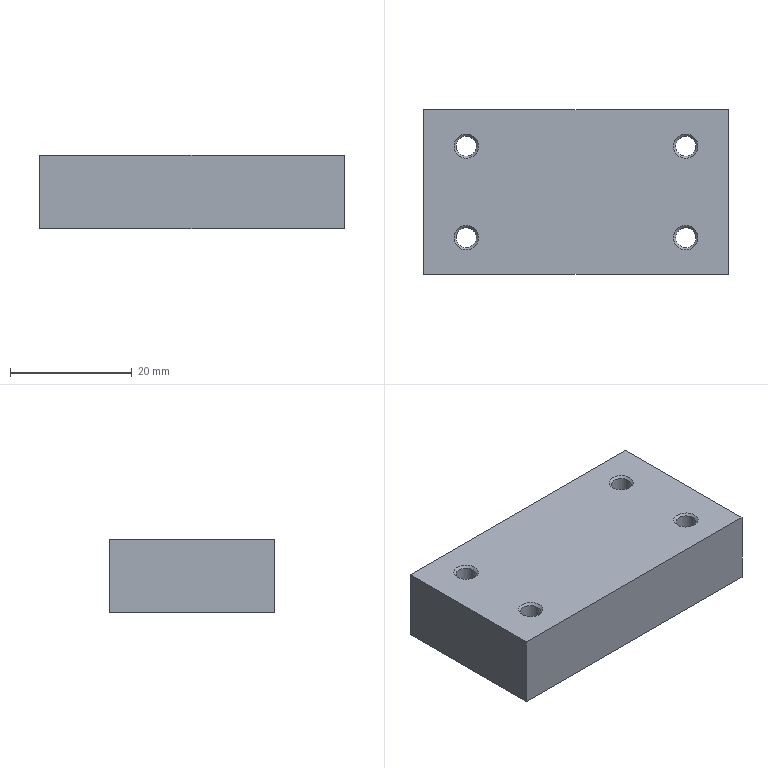Part | NX | features SIMPLE HOLE 4, SYMBOLIC_THREAD 4, DATUM_CSYS 2, BLOCK 1, HOLE PACKAGE 1, SKETCH 1 | 1 solid | 18 faces | box 50 x 27 x 12 mm | volume 15784 mm3 | cone 8 | plane 6 | cylinder 4 | commonest cylinder face diameters 3.3 x4
STEP:
#1=CARTESIAN_POINT('',(45.,21.,12.));
#2=VERTEX_POINT('',#1);
#3=CARTESIAN_POINT('',(43.,21.,12.));
#4=DIRECTION('',(0.,0.,1.));
#5=DIRECTION('',(1.,0.,0.));
#6=AXIS2_PLACEMENT_3D('',#3,#4,#5);
#7=CIRCLE('',#6,2.);
#8=EDGE_CURVE('',#2,#2,#7,.F.);
#9=ORIENTED_EDGE('',*,*,#8,.T.);
#10=EDGE_LOOP('',(#9));
#11=FACE_BOUND('',#10,.T.);
#12=CARTESIAN_POINT('',(45.,6.,12.));
#13=VERTEX_POINT('',#12);
#14=CARTESIAN_POINT('',(43.,6.,12.));
#15=DIRECTION('',(0.,0.,1.));
#16=DIRECTION('',(1.,0.,0.));
#17=AXIS2_PLACEMENT_3D('',#14,#15,#16);
#18=CIRCLE('',#17,2.);
#19=EDGE_CURVE('',#13,#13,#18,.F.);
#20=ORIENTED_EDGE('',*,*,#19,.T.);
#21=EDGE_LOOP('',(#20));
#22=FACE_BOUND('',#21,.T.);
#23=CARTESIAN_POINT('',(9.,21.,12.));
#24=VERTEX_POINT('',#23);
#25=CARTESIAN_POINT('',(7.,21.,12.));
#26=DIRECTION('',(0.,0.,1.));
#27=DIRECTION('',(1.,0.,0.));
#28=AXIS2_PLACEMENT_3D('',#25,#26,#27);
#29=CIRCLE('',#28,2.);
#30=EDGE_CURVE('',#24,#24,#29,.F.);
#31=ORIENTED_EDGE('',*,*,#30,.T.);
#32=EDGE_LOOP('',(#31));
#33=FACE_BOUND('',#32,.T.);
#34=CARTESIAN_POINT('',(9.,6.,12.));
#35=VERTEX_POINT('',#34);
#36=CARTESIAN_POINT('',(7.,6.,12.));
#37=DIRECTION('',(0.,0.,1.));
#38=DIRECTION('',(1.,0.,0.));
#39=AXIS2_PLACEMENT_3D('',#36,#37,#38);
#40=CIRCLE('',#39,2.);
#41=EDGE_CURVE('',#35,#35,#40,.F.);
#42=ORIENTED_EDGE('',*,*,#41,.T.);
#43=EDGE_LOOP('',(#42));
#44=FACE_BOUND('',#43,.T.);
#45=CARTESIAN_POINT('',(50.,0.,12.));
#46=VERTEX_POINT('',#45);
#47=CARTESIAN_POINT('',(0.,0.,12.));
#48=VERTEX_POINT('',#47);
#49=CARTESIAN_POINT('',(25.,0.,12.));
#50=DIRECTION('',(-1.,0.,0.));
#51=VECTOR('',#50,1000.);
#52=LINE('',#49,#51);
#53=EDGE_CURVE('',#46,#48,#52,.T.);
#54=ORIENTED_EDGE('',*,*,#53,.F.);
#55=CARTESIAN_POINT('',(50.,27.,12.));
#56=VERTEX_POINT('',#55);
#57=CARTESIAN_POINT('',(50.,13.5,12.));
#58=DIRECTION('',(0.,-1.,0.));
#59=VECTOR('',#58,1000.);
#60=LINE('',#57,#59);
#61=EDGE_CURVE('',#56,#46,#60,.T.);
#62=ORIENTED_EDGE('',*,*,#61,.F.);
#63=CARTESIAN_POINT('',(0.,27.,12.));
#64=VERTEX_POINT('',#63);
#65=CARTESIAN_POINT('',(25.,27.,12.));
#66=DIRECTION('',(1.,0.,0.));
#67=VECTOR('',#66,1000.);
#68=LINE('',#65,#67);
#69=EDGE_CURVE('',#64,#56,#68,.T.);
#70=ORIENTED_EDGE('',*,*,#69,.F.);
#71=CARTESIAN_POINT('',(0.,13.5,12.));
#72=DIRECTION('',(0.,1.,0.));
#73=VECTOR('',#72,1000.);
#74=LINE('',#71,#73);
#75=EDGE_CURVE('',#48,#64,#74,.T.);
#76=ORIENTED_EDGE('',*,*,#75,.F.);
#77=EDGE_LOOP('',(#54,#62,#70,#76));
#78=FACE_BOUND('',#77,.T.);
#79=CARTESIAN_POINT('',(25.,13.5,12.));
#80=DIRECTION('',(0.,0.,1.));
#81=DIRECTION('',(1.,0.,0.));
#82=AXIS2_PLACEMENT_3D('',#79,#80,#81);
#83=PLANE('',#82);
#84=ADVANCED_FACE('',(#11,#22,#33,#44,#78),#83,.T.);
#85=CARTESIAN_POINT('',(50.,0.,0.));
#86=VERTEX_POINT('',#85);
#87=CARTESIAN_POINT('',(50.,0.,0.));
#88=DIRECTION('',(0.,0.,1.));
#89=VECTOR('',#88,1000.);
#90=LINE('',#87,#89);
#91=EDGE_CURVE('',#86,#46,#90,.T.);
#92=ORIENTED_EDGE('',*,*,#91,.T.);
#93=ORIENTED_EDGE('',*,*,#53,.T.);
#94=CARTESIAN_POINT('',(0.,0.,0.));
#95=VERTEX_POINT('',#94);
#96=CARTESIAN_POINT('',(0.,0.,0.));
#97=DIRECTION('',(0.,0.,1.));
#98=VECTOR('',#97,1000.);
#99=LINE('',#96,#98);
#100=EDGE_CURVE('',#95,#48,#99,.T.);
#101=ORIENTED_EDGE('',*,*,#100,.F.);
#102=CARTESIAN_POINT('',(25.,0.,0.));
#103=DIRECTION('',(1.,0.,0.));
#104=VECTOR('',#103,1000.);
#105=LINE('',#102,#104);
#106=EDGE_CURVE('',#95,#86,#105,.T.);
#107=ORIENTED_EDGE('',*,*,#106,.T.);
#108=EDGE_LOOP('',(#92,#93,#101,#107));
#109=FACE_BOUND('',#108,.T.);
#110=CARTESIAN_POINT('',(25.,0.,0.));
#111=DIRECTION('',(0.,-1.,0.));
#112=DIRECTION('',(0.,0.,-1.));
#113=AXIS2_PLACEMENT_3D('',#110,#111,#112);
#114=PLANE('',#113);
#115=ADVANCED_FACE('',(#109),#114,.T.);
#116=ORIENTED_EDGE('',*,*,#100,.T.);
#117=ORIENTED_EDGE('',*,*,#75,.T.);
#118=CARTESIAN_POINT('',(0.,27.,0.));
#119=VERTEX_POINT('',#118);
#120=CARTESIAN_POINT('',(0.,27.,0.));
#121=DIRECTION('',(0.,0.,1.));
#122=VECTOR('',#121,1000.);
#123=LINE('',#120,#122);
#124=EDGE_CURVE('',#119,#64,#123,.T.);
#125=ORIENTED_EDGE('',*,*,#124,.F.);
#126=CARTESIAN_POINT('',(0.,13.5,0.));
#127=DIRECTION('',(0.,-1.,0.));
#128=VECTOR('',#127,1000.);
#129=LINE('',#126,#128);
#130=EDGE_CURVE('',#119,#95,#129,.T.);
#131=ORIENTED_EDGE('',*,*,#130,.T.);
#132=EDGE_LOOP('',(#116,#117,#125,#131));
#133=FACE_BOUND('',#132,.T.);
#134=CARTESIAN_POINT('',(0.,13.5,0.));
#135=DIRECTION('',(-1.,0.,0.));
#136=DIRECTION('',(0.,0.,1.));
#137=AXIS2_PLACEMENT_3D('',#134,#135,#136);
#138=PLANE('',#137);
#139=ADVANCED_FACE('',(#133),#138,.T.);
#140=ORIENTED_EDGE('',*,*,#124,.T.);
#141=ORIENTED_EDGE('',*,*,#69,.T.);
#142=CARTESIAN_POINT('',(50.,27.,0.));
#143=VERTEX_POINT('',#142);
#144=CARTESIAN_POINT('',(50.,27.,0.));
#145=DIRECTION('',(0.,0.,1.));
#146=VECTOR('',#145,1000.);
#147=LINE('',#144,#146);
#148=EDGE_CURVE('',#143,#56,#147,.T.);
#149=ORIENTED_EDGE('',*,*,#148,.F.);
#150=CARTESIAN_POINT('',(25.,27.,0.));
#151=DIRECTION('',(-1.,0.,0.));
#152=VECTOR('',#151,1000.);
#153=LINE('',#150,#152);
#154=EDGE_CURVE('',#143,#119,#153,.T.);
#155=ORIENTED_EDGE('',*,*,#154,.T.);
#156=EDGE_LOOP('',(#140,#141,#149,#155));
#157=FACE_BOUND('',#156,.T.);
#158=CARTESIAN_POINT('',(25.,27.,0.));
#159=DIRECTION('',(0.,1.,0.));
#160=DIRECTION('',(0.,0.,1.));
#161=AXIS2_PLACEMENT_3D('',#158,#159,#160);
#162=PLANE('',#161);
#163=ADVANCED_FACE('',(#157),#162,.T.);
#164=CARTESIAN_POINT('',(41.,21.,0.));
#165=VERTEX_POINT('',#164);
#166=CARTESIAN_POINT('',(43.,21.,0.));
#167=DIRECTION('',(0.,0.,-1.));
#168=DIRECTION('',(-1.,0.,0.));
#169=AXIS2_PLACEMENT_3D('',#166,#167,#168);
#170=CIRCLE('',#169,2.);
#171=EDGE_CURVE('',#165,#165,#170,.F.);
#172=ORIENTED_EDGE('',*,*,#171,.T.);
#173=EDGE_LOOP('',(#172));
#174=FACE_BOUND('',#173,.T.);
#175=CARTESIAN_POINT('',(41.,6.,0.));
#176=VERTEX_POINT('',#175);
#177=CARTESIAN_POINT('',(43.,6.,0.));
#178=DIRECTION('',(0.,0.,-1.));
#179=DIRECTION('',(-1.,0.,0.));
#180=AXIS2_PLACEMENT_3D('',#177,#178,#179);
#181=CIRCLE('',#180,2.);
#182=EDGE_CURVE('',#176,#176,#181,.F.);
#183=ORIENTED_EDGE('',*,*,#182,.T.);
#184=EDGE_LOOP('',(#183));
#185=FACE_BOUND('',#184,.T.);
#186=CARTESIAN_POINT('',(5.,21.,0.));
#187=VERTEX_POINT('',#186);
#188=CARTESIAN_POINT('',(7.,21.,0.));
#189=DIRECTION('',(0.,0.,-1.));
#190=DIRECTION('',(-1.,0.,0.));
#191=AXIS2_PLACEMENT_3D('',#188,#189,#190);
#192=CIRCLE('',#191,2.);
#193=EDGE_CURVE('',#187,#187,#192,.F.);
#194=ORIENTED_EDGE('',*,*,#193,.T.);
#195=EDGE_LOOP('',(#194));
#196=FACE_BOUND('',#195,.T.);
#197=CARTESIAN_POINT('',(5.,6.,0.));
#198=VERTEX_POINT('',#197);
#199=CARTESIAN_POINT('',(7.,6.,0.));
#200=DIRECTION('',(0.,0.,-1.));
#201=DIRECTION('',(-1.,0.,0.));
#202=AXIS2_PLACEMENT_3D('',#199,#200,#201);
#203=CIRCLE('',#202,2.);
#204=EDGE_CURVE('',#198,#198,#203,.F.);
#205=ORIENTED_EDGE('',*,*,#204,.T.);
#206=EDGE_LOOP('',(#205));
#207=FACE_BOUND('',#206,.T.);
#208=CARTESIAN_POINT('',(50.,13.5,0.));
#209=DIRECTION('',(0.,1.,0.));
#210=VECTOR('',#209,1000.);
#211=LINE('',#208,#210);
#212=EDGE_CURVE('',#86,#143,#211,.T.);
#213=ORIENTED_EDGE('',*,*,#212,.F.);
#214=ORIENTED_EDGE('',*,*,#106,.F.);
#215=ORIENTED_EDGE('',*,*,#130,.F.);
#216=ORIENTED_EDGE('',*,*,#154,.F.);
#217=EDGE_LOOP('',(#213,#214,#215,#216));
#218=FACE_BOUND('',#217,.T.);
#219=CARTESIAN_POINT('',(25.,13.5,0.));
#220=DIRECTION('',(0.,0.,-1.));
#221=DIRECTION('',(-1.,0.,0.));
#222=AXIS2_PLACEMENT_3D('',#219,#220,#221);
#223=PLANE('',#222);
#224=ADVANCED_FACE('',(#174,#185,#196,#207,#218),#223,.T.);
#225=ORIENTED_EDGE('',*,*,#212,.T.);
#226=ORIENTED_EDGE('',*,*,#148,.T.);
#227=ORIENTED_EDGE('',*,*,#61,.T.);
#228=ORIENTED_EDGE('',*,*,#91,.F.);
#229=EDGE_LOOP('',(#225,#226,#227,#228));
#230=FACE_BOUND('',#229,.T.);
#231=CARTESIAN_POINT('',(50.,13.5,0.));
#232=DIRECTION('',(1.,0.,0.));
#233=DIRECTION('',(0.,0.,-1.));
#234=AXIS2_PLACEMENT_3D('',#231,#232,#233);
#235=PLANE('',#234);
#236=ADVANCED_FACE('',(#230),#235,.T.);
#237=CARTESIAN_POINT('',(5.35,6.,0.35));
#238=VERTEX_POINT('',#237);
#239=CARTESIAN_POINT('',(7.,6.,0.35));
#240=DIRECTION('',(0.,0.,-1.));
#241=DIRECTION('',(-1.,0.,0.));
#242=AXIS2_PLACEMENT_3D('',#239,#240,#241);
#243=CIRCLE('',#242,1.65);
#244=EDGE_CURVE('',#238,#238,#243,.T.);
#245=ORIENTED_EDGE('',*,*,#244,.T.);
#246=EDGE_LOOP('',(#245));
#247=FACE_BOUND('',#246,.T.);
#248=CARTESIAN_POINT('',(8.65,6.,11.65));
#249=VERTEX_POINT('',#248);
#250=CARTESIAN_POINT('',(7.,6.,11.65));
#251=DIRECTION('',(0.,0.,1.));
#252=DIRECTION('',(1.,0.,0.));
#253=AXIS2_PLACEMENT_3D('',#250,#251,#252);
#254=CIRCLE('',#253,1.65);
#255=EDGE_CURVE('',#249,#249,#254,.T.);
#256=ORIENTED_EDGE('',*,*,#255,.T.);
#257=EDGE_LOOP('',(#256));
#258=FACE_BOUND('',#257,.T.);
#259=CARTESIAN_POINT('',(7.,6.,12.));
#260=DIRECTION('',(0.,0.,-1.));
#261=DIRECTION('',(-1.,0.,0.));
#262=AXIS2_PLACEMENT_3D('',#259,#260,#261);
#263=CYLINDRICAL_SURFACE('',#262,1.65);
#264=ADVANCED_FACE('',(#247,#258),#263,.F.);
#265=ORIENTED_EDGE('',*,*,#255,.F.);
#266=EDGE_LOOP('',(#265));
#267=FACE_BOUND('',#266,.T.);
#268=ORIENTED_EDGE('',*,*,#41,.F.);
#269=EDGE_LOOP('',(#268));
#270=FACE_BOUND('',#269,.T.);
#271=CARTESIAN_POINT('',(7.,6.,12.));
#272=DIRECTION('',(0.,0.,1.));
#273=DIRECTION('',(1.,0.,0.));
#274=AXIS2_PLACEMENT_3D('',#271,#272,#273);
#275=CONICAL_SURFACE('',#274,2.,0.7854);
#276=ADVANCED_FACE('',(#267,#270),#275,.F.);
#277=ORIENTED_EDGE('',*,*,#204,.F.);
#278=EDGE_LOOP('',(#277));
#279=FACE_BOUND('',#278,.T.);
#280=ORIENTED_EDGE('',*,*,#244,.F.);
#281=EDGE_LOOP('',(#280));
#282=FACE_BOUND('',#281,.T.);
#283=CARTESIAN_POINT('',(7.,6.,0.35));
#284=DIRECTION('',(0.,0.,-1.));
#285=DIRECTION('',(-1.,0.,0.));
#286=AXIS2_PLACEMENT_3D('',#283,#284,#285);
#287=CONICAL_SURFACE('',#286,1.65,0.7854);
#288=ADVANCED_FACE('',(#279,#282),#287,.F.);
#289=CARTESIAN_POINT('',(5.35,21.,0.35));
#290=VERTEX_POINT('',#289);
#291=CARTESIAN_POINT('',(7.,21.,0.35));
#292=DIRECTION('',(0.,0.,-1.));
#293=DIRECTION('',(-1.,0.,0.));
#294=AXIS2_PLACEMENT_3D('',#291,#292,#293);
#295=CIRCLE('',#294,1.65);
#296=EDGE_CURVE('',#290,#290,#295,.T.);
#297=ORIENTED_EDGE('',*,*,#296,.T.);
#298=EDGE_LOOP('',(#297));
#299=FACE_BOUND('',#298,.T.);
#300=CARTESIAN_POINT('',(8.65,21.,11.65));
#301=VERTEX_POINT('',#300);
#302=CARTESIAN_POINT('',(7.,21.,11.65));
#303=DIRECTION('',(0.,0.,1.));
#304=DIRECTION('',(1.,0.,0.));
#305=AXIS2_PLACEMENT_3D('',#302,#303,#304);
#306=CIRCLE('',#305,1.65);
#307=EDGE_CURVE('',#301,#301,#306,.T.);
#308=ORIENTED_EDGE('',*,*,#307,.T.);
#309=EDGE_LOOP('',(#308));
#310=FACE_BOUND('',#309,.T.);
#311=CARTESIAN_POINT('',(7.,21.,12.));
#312=DIRECTION('',(0.,0.,-1.));
#313=DIRECTION('',(-1.,0.,0.));
#314=AXIS2_PLACEMENT_3D('',#311,#312,#313);
#315=CYLINDRICAL_SURFACE('',#314,1.65);
#316=ADVANCED_FACE('',(#299,#310),#315,.F.);
#317=ORIENTED_EDGE('',*,*,#307,.F.);
#318=EDGE_LOOP('',(#317));
#319=FACE_BOUND('',#318,.T.);
#320=ORIENTED_EDGE('',*,*,#30,.F.);
#321=EDGE_LOOP('',(#320));
#322=FACE_BOUND('',#321,.T.);
#323=CARTESIAN_POINT('',(7.,21.,12.));
#324=DIRECTION('',(0.,0.,1.));
#325=DIRECTION('',(1.,0.,0.));
#326=AXIS2_PLACEMENT_3D('',#323,#324,#325);
#327=CONICAL_SURFACE('',#326,2.,0.7854);
#328=ADVANCED_FACE('',(#319,#322),#327,.F.);
#329=ORIENTED_EDGE('',*,*,#193,.F.);
#330=EDGE_LOOP('',(#329));
#331=FACE_BOUND('',#330,.T.);
#332=ORIENTED_EDGE('',*,*,#296,.F.);
#333=EDGE_LOOP('',(#332));
#334=FACE_BOUND('',#333,.T.);
#335=CARTESIAN_POINT('',(7.,21.,0.35));
#336=DIRECTION('',(0.,0.,-1.));
#337=DIRECTION('',(-1.,0.,0.));
#338=AXIS2_PLACEMENT_3D('',#335,#336,#337);
#339=CONICAL_SURFACE('',#338,1.65,0.7854);
#340=ADVANCED_FACE('',(#331,#334),#339,.F.);
#341=CARTESIAN_POINT('',(41.35,6.,0.35));
#342=VERTEX_POINT('',#341);
#343=CARTESIAN_POINT('',(43.,6.,0.35));
#344=DIRECTION('',(0.,0.,-1.));
#345=DIRECTION('',(-1.,0.,0.));
#346=AXIS2_PLACEMENT_3D('',#343,#344,#345);
#347=CIRCLE('',#346,1.65);
#348=EDGE_CURVE('',#342,#342,#347,.T.);
#349=ORIENTED_EDGE('',*,*,#348,.T.);
#350=EDGE_LOOP('',(#349));
#351=FACE_BOUND('',#350,.T.);
#352=CARTESIAN_POINT('',(44.65,6.,11.65));
#353=VERTEX_POINT('',#352);
#354=CARTESIAN_POINT('',(43.,6.,11.65));
#355=DIRECTION('',(0.,0.,1.));
#356=DIRECTION('',(1.,0.,0.));
#357=AXIS2_PLACEMENT_3D('',#354,#355,#356);
#358=CIRCLE('',#357,1.65);
#359=EDGE_CURVE('',#353,#353,#358,.T.);
#360=ORIENTED_EDGE('',*,*,#359,.T.);
#361=EDGE_LOOP('',(#360));
#362=FACE_BOUND('',#361,.T.);
#363=CARTESIAN_POINT('',(43.,6.,12.));
#364=DIRECTION('',(0.,0.,-1.));
#365=DIRECTION('',(-1.,0.,0.));
#366=AXIS2_PLACEMENT_3D('',#363,#364,#365);
#367=CYLINDRICAL_SURFACE('',#366,1.65);
#368=ADVANCED_FACE('',(#351,#362),#367,.F.);
#369=ORIENTED_EDGE('',*,*,#359,.F.);
#370=EDGE_LOOP('',(#369));
#371=FACE_BOUND('',#370,.T.);
#372=ORIENTED_EDGE('',*,*,#19,.F.);
#373=EDGE_LOOP('',(#372));
#374=FACE_BOUND('',#373,.T.);
#375=CARTESIAN_POINT('',(43.,6.,12.));
#376=DIRECTION('',(0.,0.,1.));
#377=DIRECTION('',(1.,0.,0.));
#378=AXIS2_PLACEMENT_3D('',#375,#376,#377);
#379=CONICAL_SURFACE('',#378,2.,0.7854);
#380=ADVANCED_FACE('',(#371,#374),#379,.F.);
#381=ORIENTED_EDGE('',*,*,#182,.F.);
#382=EDGE_LOOP('',(#381));
#383=FACE_BOUND('',#382,.T.);
#384=ORIENTED_EDGE('',*,*,#348,.F.);
#385=EDGE_LOOP('',(#384));
#386=FACE_BOUND('',#385,.T.);
#387=CARTESIAN_POINT('',(43.,6.,0.35));
#388=DIRECTION('',(0.,0.,-1.));
#389=DIRECTION('',(-1.,0.,0.));
#390=AXIS2_PLACEMENT_3D('',#387,#388,#389);
#391=CONICAL_SURFACE('',#390,1.65,0.7854);
#392=ADVANCED_FACE('',(#383,#386),#391,.F.);
#393=CARTESIAN_POINT('',(41.35,21.,0.35));
#394=VERTEX_POINT('',#393);
#395=CARTESIAN_POINT('',(43.,21.,0.35));
#396=DIRECTION('',(0.,0.,-1.));
#397=DIRECTION('',(-1.,0.,0.));
#398=AXIS2_PLACEMENT_3D('',#395,#396,#397);
#399=CIRCLE('',#398,1.65);
#400=EDGE_CURVE('',#394,#394,#399,.T.);
#401=ORIENTED_EDGE('',*,*,#400,.T.);
#402=EDGE_LOOP('',(#401));
#403=FACE_BOUND('',#402,.T.);
#404=CARTESIAN_POINT('',(44.65,21.,11.65));
#405=VERTEX_POINT('',#404);
#406=CARTESIAN_POINT('',(43.,21.,11.65));
#407=DIRECTION('',(0.,0.,1.));
#408=DIRECTION('',(1.,0.,0.));
#409=AXIS2_PLACEMENT_3D('',#406,#407,#408);
#410=CIRCLE('',#409,1.65);
#411=EDGE_CURVE('',#405,#405,#410,.T.);
#412=ORIENTED_EDGE('',*,*,#411,.T.);
#413=EDGE_LOOP('',(#412));
#414=FACE_BOUND('',#413,.T.);
#415=CARTESIAN_POINT('',(43.,21.,12.));
#416=DIRECTION('',(0.,0.,-1.));
#417=DIRECTION('',(-1.,0.,0.));
#418=AXIS2_PLACEMENT_3D('',#415,#416,#417);
#419=CYLINDRICAL_SURFACE('',#418,1.65);
#420=ADVANCED_FACE('',(#403,#414),#419,.F.);
#421=ORIENTED_EDGE('',*,*,#411,.F.);
#422=EDGE_LOOP('',(#421));
#423=FACE_BOUND('',#422,.T.);
#424=ORIENTED_EDGE('',*,*,#8,.F.);
#425=EDGE_LOOP('',(#424));
#426=FACE_BOUND('',#425,.T.);
#427=CARTESIAN_POINT('',(43.,21.,12.));
#428=DIRECTION('',(0.,0.,1.));
#429=DIRECTION('',(1.,0.,0.));
#430=AXIS2_PLACEMENT_3D('',#427,#428,#429);
#431=CONICAL_SURFACE('',#430,2.,0.7854);
#432=ADVANCED_FACE('',(#423,#426),#431,.F.);
#433=ORIENTED_EDGE('',*,*,#171,.F.);
#434=EDGE_LOOP('',(#433));
#435=FACE_BOUND('',#434,.T.);
#436=ORIENTED_EDGE('',*,*,#400,.F.);
#437=EDGE_LOOP('',(#436));
#438=FACE_BOUND('',#437,.T.);
#439=CARTESIAN_POINT('',(43.,21.,0.35));
#440=DIRECTION('',(0.,0.,-1.));
#441=DIRECTION('',(-1.,0.,0.));
#442=AXIS2_PLACEMENT_3D('',#439,#440,#441);
#443=CONICAL_SURFACE('',#442,1.65,0.7854);
#444=ADVANCED_FACE('',(#435,#438),#443,.F.);
#445=CLOSED_SHELL('',(#84,#115,#139,#163,#224,#236,#264,#276,#288,#316,#328,#340,#368,#380,#392,#420,#432,#444));
#446=MANIFOLD_SOLID_BREP('',#445);
#447=(LENGTH_UNIT()NAMED_UNIT(*)SI_UNIT(.MILLI.,.METRE.));
#448=UNCERTAINTY_MEASURE_WITH_UNIT(LENGTH_MEASURE(0.00001),#447,'','');
#449=(NAMED_UNIT(*)PLANE_ANGLE_UNIT()SI_UNIT($,.RADIAN.));
#450=(NAMED_UNIT(*)SI_UNIT($,.STERADIAN.)SOLID_ANGLE_UNIT());
#451=(GEOMETRIC_REPRESENTATION_CONTEXT(3)GLOBAL_UNCERTAINTY_ASSIGNED_CONTEXT((#448))GLOBAL_UNIT_ASSIGNED_CONTEXT((#447,#449,#450))REPRESENTATION_CONTEXT('',''));
#452=ADVANCED_BREP_SHAPE_REPRESENTATION('',(#446),#451);